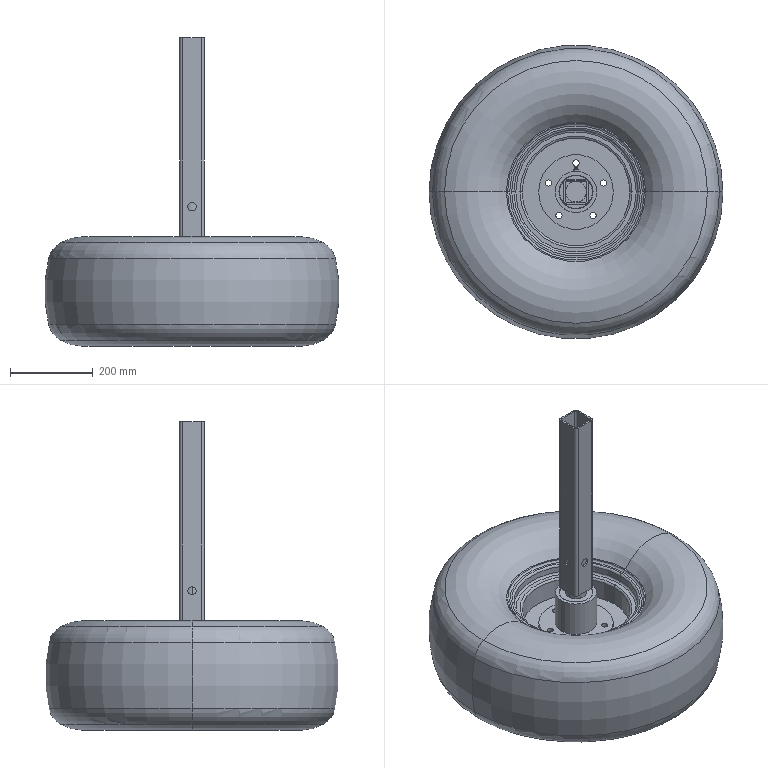Part | SolidWorks | features CompositeCurve 25, Cut 1 | 46 solids | 770 faces | box 710 x 710 x 743.5 mm | volume 77284937 mm3 | cylinder 317 | plane 169 | sphere 132 | torus 90 | cone 62 | commonest cylinder face diameters 58 x58 62 x58 15 x20 8 x19 5 x16 53.333 x16